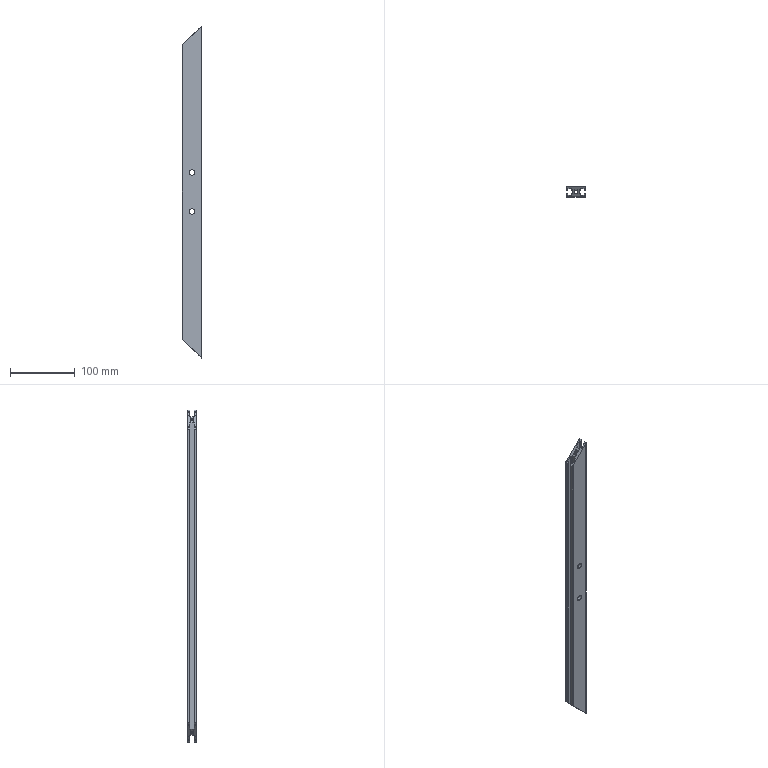Part | NX | features BREP 1 | 1 solid | 127 faces | box 30 x 15 x 512.1 mm | volume 114716 mm3 | cylinder 65 | plane 54 | cone 8 | commonest cylinder face diameters 5 x23 1 x18 3.3 x16 2 x4 8.5 x4